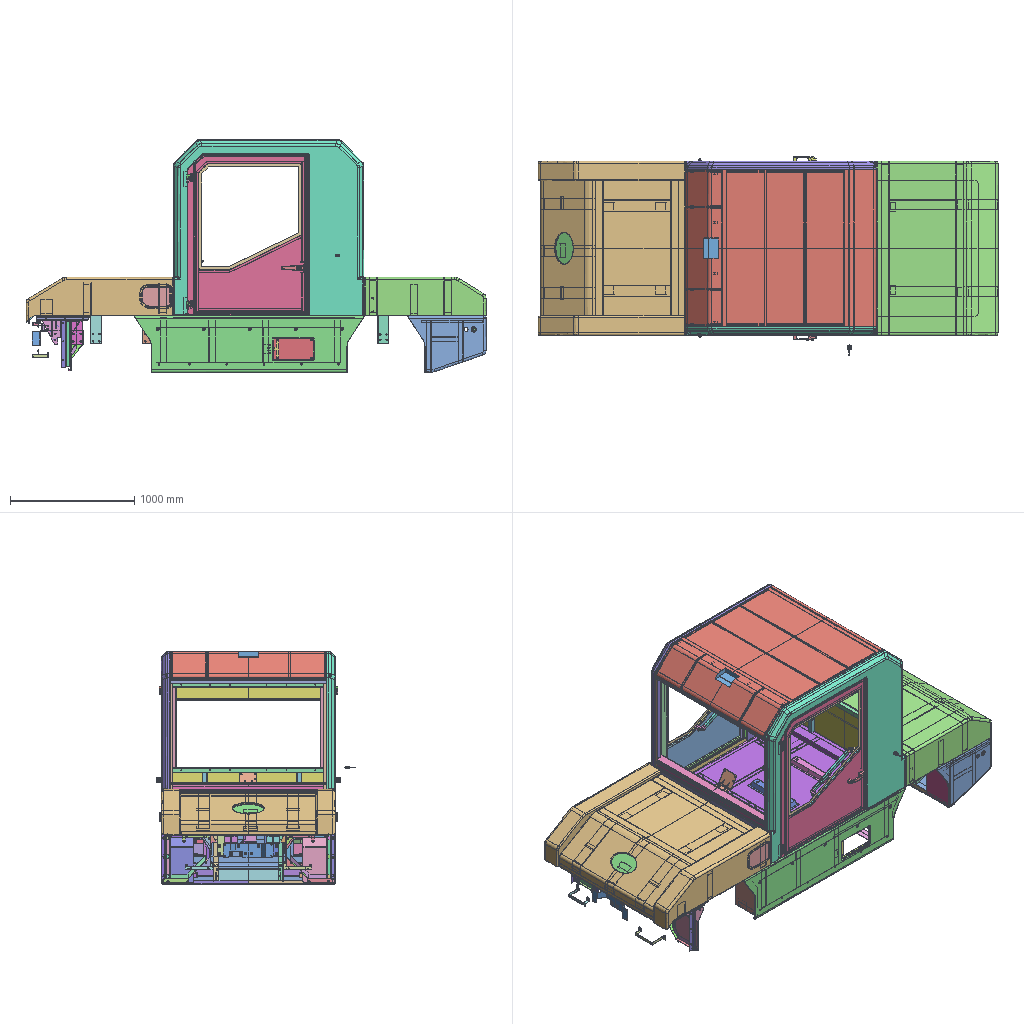Assembly | NX | 146 different items | 266 placed | box 3700 x 1601 x 1871 mm
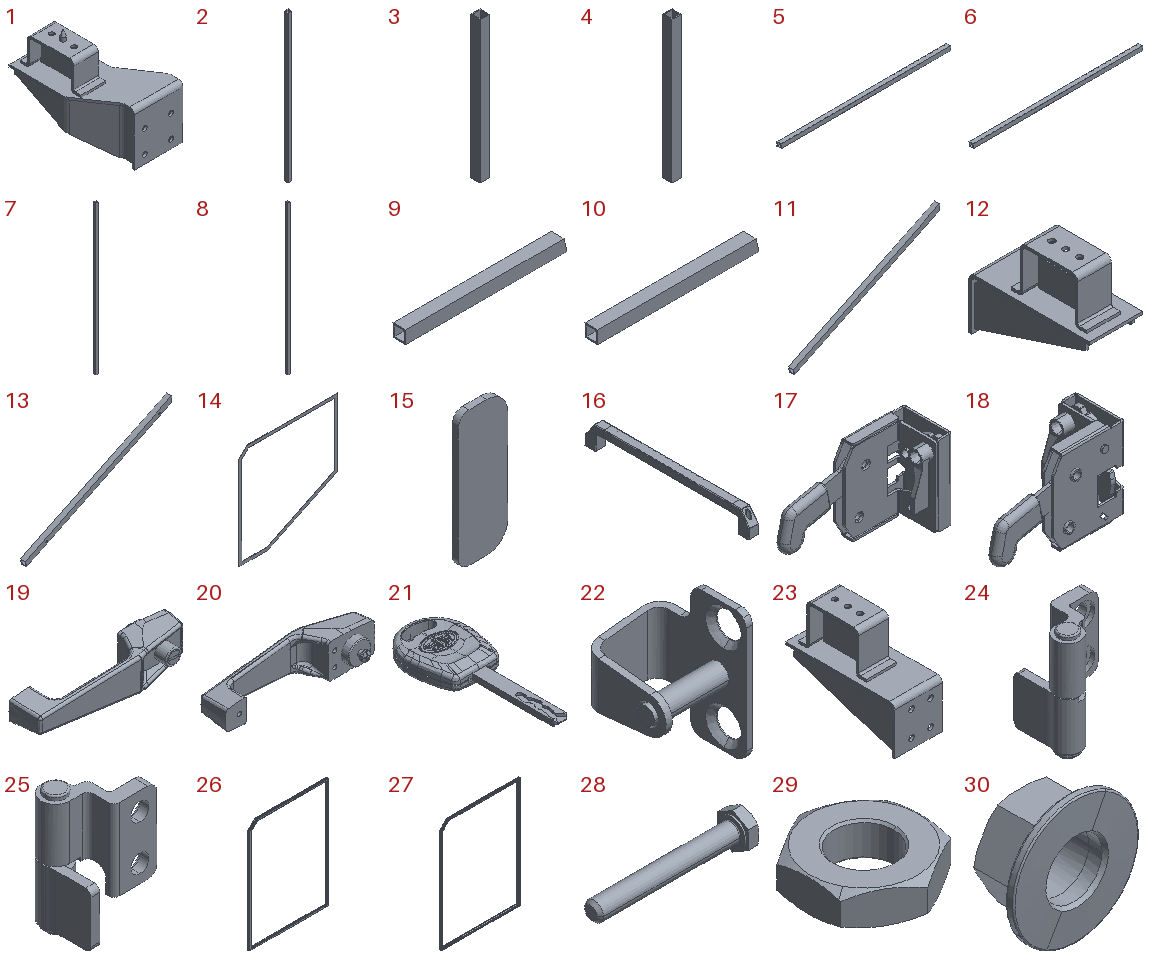Parts list (item | quantity | parent item | size | volume | features):
1 | x1 | in 92 | 193 x 272 x 240 mm | 719296 mm3 | features BREP 7
2 | x1 | in 134 | 20 x 20 x 807.958 mm | 116344 mm3 | features BREP 1
3 | x1 | in 133 | 20 x 20 x 309.106 mm | 44509 mm3 | features BREP 1
4 | x1 | in 134 | 20 x 20 x 309.106 mm | 44509 mm3 | features BREP 1
5 | x1 | in 133 | 830.914 x 20 x 20 mm | 119652 mm3 | features BREP 1
6 | x1 | in 134 | 830.914 x 20 x 20 mm | 119652 mm3 | features BREP 1
7 | x1 | in 133 | - | 161028 mm3 | features BREP 1
8 | x1 | in 134 | 20 x 20 x 1122 mm | 161028 mm3 | features BREP 1
9 | x1 | in 133 | 252.949 x 20 x 20 mm | 36094 mm3 | features BREP 1
10 | x1 | in 134 | 252.949 x 20 x 20 mm | 36094 mm3 | features BREP 1
11 | x1 | in 133 | - | 92693 mm3 | features BREP 1
12 | x1 | in 92 | 114 x 260 x 212 mm | 600917 mm3 | features BREP 6
13 | x1 | in 134 | - | 92693 mm3 | features BREP 1
14 | x2 | in 133, 134 | 830.914 x 2 x 852.689 mm | 150814 mm3 | features BREP 1
15 | x4 | in 133, 134 | - | 4337 mm3 | features BREP 1
16 | x2 | in 135 | 35.311 x 535.2 x 70.2 mm | 135109 mm3 | features BREP 3
17 | x1 | in 135 | 115.249 x 44.6 x 74.6 mm | 46344 mm3 | features BREP 15
18 | x1 | in 135 | - | - | features BREP 15
19 | x1 | in 135 | 184.421 x 56.842 x 42.453 mm | 116707 mm3 | features BREP 1
20 | x1 | in 135 | - | - | features BREP 1
21 | x1 | in 135 | 32.729 x 84.992 x 10.488 mm | 6335 mm3 | features BREP 3
22 | x2 | in 135 | 37 x 44.176 x 60 mm | 11849 mm3 | features BREP 2
23 | x1 | in 92 | 114 x 260 x 212 mm | 600917 mm3 | features BREP 6
24 | x2 | in 135 | 42 x 34.8 x 68 mm | 24506 mm3 | features BREP 6
25 | x2 | in 135 | - | - | features BREP 6
26 | x1 | in 135 | 921.878 x 23.5 x 1292 mm | 1729041 mm3 | features BREP 40
27 | x1 | in 135 | - | - | features BREP 20
28 | x4 | in 135 | 49 x 10 x 11.547 mm | 1597 mm3 | features BREP 1
29 | x8 | in 135 | 13 x 15.011 x 4 mm | 421.241 mm3 | features BREP 1
30 | x6 | in 12, 23, 125 | 26 x 11.959 x 26 mm | 2329 mm3 | features BREP 1
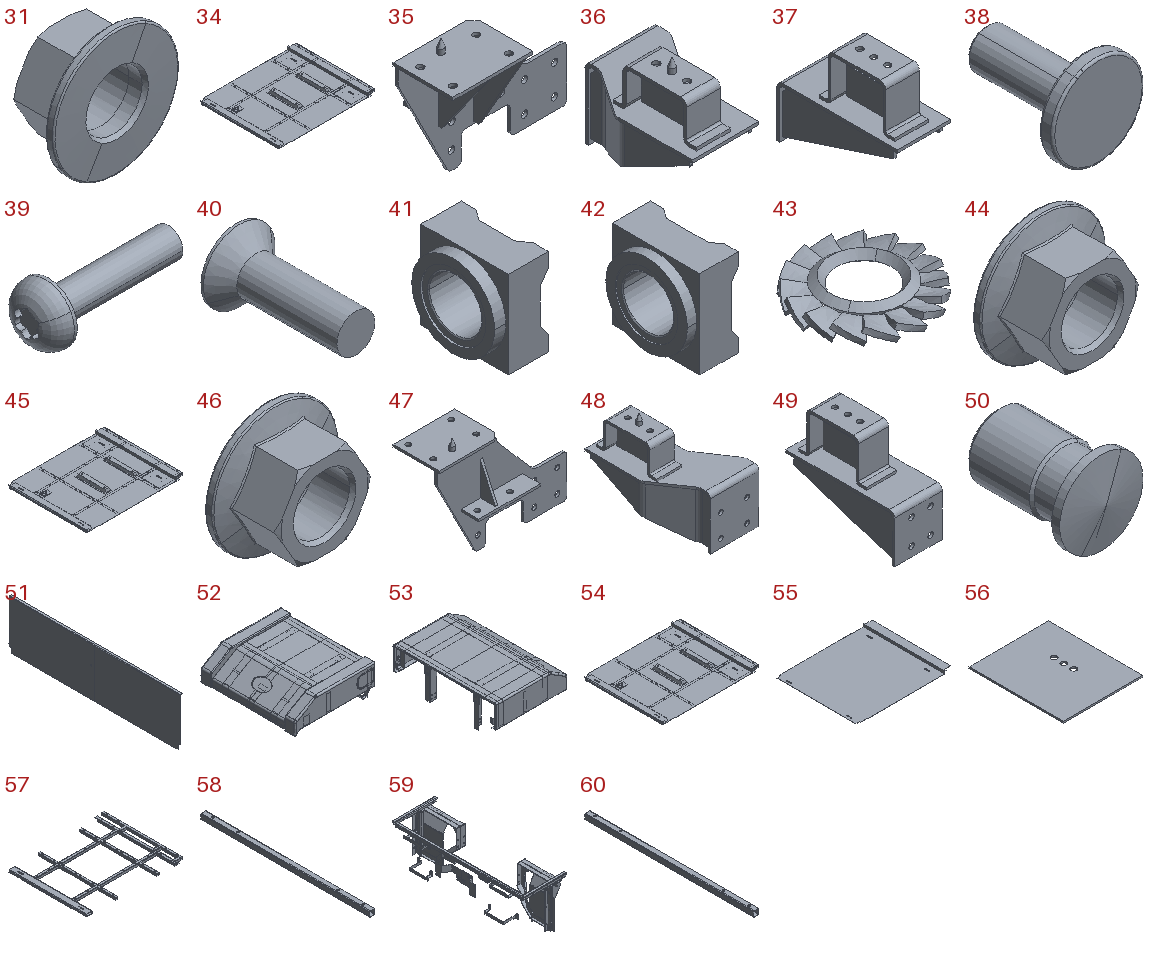31 | x4 | in 114 | 26 x 11.959 x 26 mm | 2329 mm3 | features BREP 1
32 | x1 | in 92 | - | - | -
33 | x1 | in 81 | - | - | -
34 | x1 | in 103 | 1524 x 1300 x 84.135 mm | 9485940 mm3 | features BREP 16
35 | x1 | in 114 | 337.5 x 161 x 259 mm | 536399 mm3 | features BREP 7
36 | x1 | in 125 | 193 x 272 x 240 mm | 714638 mm3 | features BREP 6
37 | x1 | in 12 | 114 x 260 x 212 mm | 596260 mm3 | features BREP 5
38 | x3 | in 73 | 18.5 x 22.7 x 18.5 mm | 1736 mm3 | features BREP 1
39 | x10 | in 135 | 29.6 x 12 x 12 mm | 1095 mm3 | features BREP 1
40 | x4 | in 135 | 15 x 25 x 15 mm | 1509 mm3 | features BREP 1
41 | x4 | in 133, 134 | 5.9 x 10 x 10 mm | 326.565 mm3 | features BREP 1
42 | x14 | in 64, 65, 82, 84, 95, 96, 100 | 7.6 x 14 x 14 mm | 863.218 mm3 | features BREP 1
43 | x4 | in 135 | 16.312 x 16.312 x 2.545 mm | 132.852 mm3 | features BREP 1
44 | x2 | in 1 | 26 x 11.959 x 26 mm | 2329 mm3 | features BREP 1
45 | x1 | in 34 | 1524 x 1300 x 84.135 mm | 9485940 mm3 | features BREP 16
46 | x4 | in 136 | 26 x 11.959 x 26 mm | 2329 mm3 | features BREP 1
47 | x1 | in 136 | 337.5 x 161 x 259 mm | 536399 mm3 | features BREP 7
48 | x1 | in 1 | 193 x 272 x 240 mm | 714638 mm3 | features BREP 6
49 | x1 | in 23 | 114 x 260 x 212 mm | 596260 mm3 | features BREP 5
50 | x8 | in 133, 134 | 10.4 x 13.638 x 10.4 mm | 676.067 mm3 | features BREP 1
51 | x1 | in 84 | 20 x 1258 x 356.004 mm | 935299 mm3 | features BREP 1
52 | x1 | - | 1184 x 1400 x 540.004 mm | 11251128 mm3 | features BREP 91
53 | x1 | - | 983.421 x 1400 x 533.004 mm | 8293382 mm3 | features BREP 71
54 | x1 | in 45 | 1524 x 1300 x 84.135 mm | 9485940 mm3 | features BREP 16
55 | x1 | in 54 | 1516 x 1300 x 44 mm | 4032528 mm3 | features BREP 1
56 | x2 | in 54 | 243.37 x 288 x 5 mm | 347049 mm3 | features BREP 1
57 | x1 | in 54 | 1524 x 1300 x 82 mm | 3863519 mm3 | features BREP 8
58 | x1 | in 57 | 40 x 1258 x 40 mm | 362402 mm3 | features BREP 1
59 | x1 | in 76 | 460.374 x 1390 x 435 mm | 2769143 mm3 | features BREP 60
60 | x1 | in 57 | 40 x 1225 x 40 mm | 352740 mm3 | features BREP 1
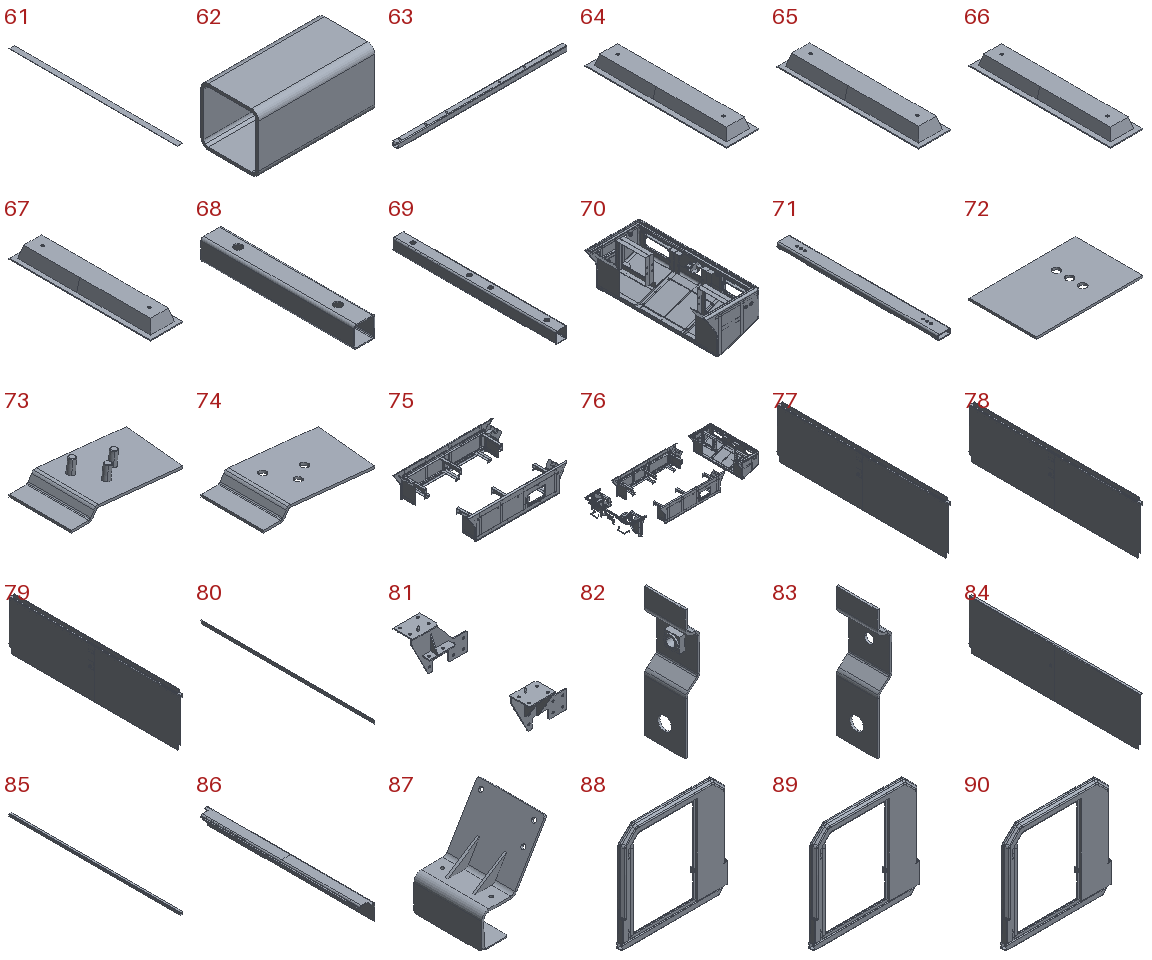61 | x1 | in 57 | 40 x 1300 x 2 mm | 104000 mm3 | features BREP 1
62 | x4 | in 57 | 80.5 x 40 x 40 mm | 23366 mm3 | features BREP 1
63 | x2 | in 57 | 1303 x 40 x 40 mm | 373746 mm3 | features BREP 1
64 | x1 | in 54 | 110 x 481.5 x 37.13 mm | 239621 mm3 | features BREP 2
65 | x1 | in 54 | 110 x 481.5 x 42.13 mm | 251733 mm3 | features BREP 2
66 | x1 | in 64 | 110 x 481.5 x 37.13 mm | 237895 mm3 | features BREP 1
67 | x1 | in 65 | 110 x 481.5 x 42.13 mm | 250007 mm3 | features BREP 1
68 | x4 | in 57 | 40 x 288 x 40 mm | 82180 mm3 | features BREP 1
69 | x2 | in 57 | 40 x 568.999 x 40 mm | 162331 mm3 | features BREP 1
70 | x1 | in 76 | 632.819 x 1400 x 457 mm | 1445450 mm3 | features BREP 93
71 | x1 | in 57 | 100.003 x 1225 x 40 mm | 1550034 mm3 | features BREP 1
72 | x2 | in 54 | 243.374 x 152.848 x 5 mm | 182593 mm3 | features BREP 1
73 | x1 | in 54 | 145.982 x 77.757 x 29.86 mm | 39257 mm3 | features BREP 2
74 | x1 | in 73 | 145.982 x 77.757 x 14.741 mm | 34048 mm3 | features BREP 1
75 | x1 | in 76 | 1856 x 1400 x 457 mm | 7771969 mm3 | features BREP 109
76 | x1 | - | - | 31583893 mm3 | features BREP 278
77 | x1 | in 103 | 28.499 x 1258 x 378.001 mm | 1221396 mm3 | features BREP 5
78 | x1 | in 77 | 28.499 x 1258 x 378.001 mm | 1221396 mm3 | features BREP 5
79 | x1 | in 78 | 28.499 x 1258 x 378.001 mm | 1221396 mm3 | features BREP 5
80 | x1 | in 79 | 4 x 1214 x 21.997 mm | 106850 mm3 | features BREP 1
81 | x1 | in 76 | 337.5 x 830 x 259 mm | 1091429 mm3 | features BREP 16
82 | x1 | in 79 | 14 x 39 x 122.887 mm | 10991 mm3 | features BREP 2
83 | x1 | in 82 | 14 x 39 x 122.887 mm | 10128 mm3 | features BREP 1
84 | x1 | in 79 | 26.5 x 1258 x 356.004 mm | 936162 mm3 | features BREP 2
85 | x1 | in 79 | 20 x 1258 x 20 mm | 167394 mm3 | features BREP 1
86 | x1 | - | 98.003 x 1318 x 131 mm | 1286068 mm3 | features BREP 2
87 | x1 | - | 135.55 x 140 x 179.776 mm | 207099 mm3 | features BREP 2
88 | x1 | in 103 | 1528 x 92.834 x 1503 mm | 9597800 mm3 | features BREP 10
89 | x1 | in 88 | 1528 x 92.834 x 1503 mm | 9597800 mm3 | features BREP 10
90 | x1 | in 89 | 1528 x 92.834 x 1503 mm | 9597800 mm3 | features BREP 10
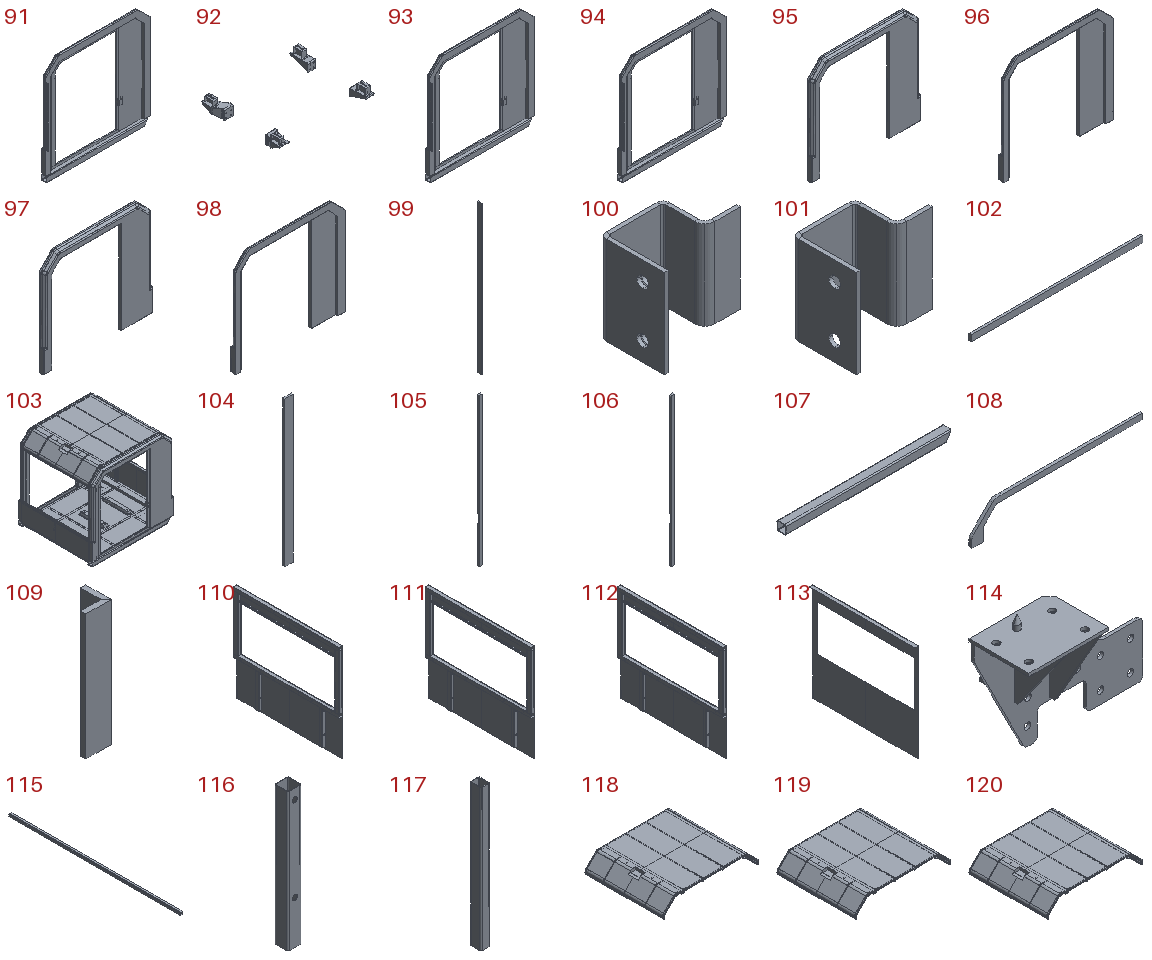91 | x1 | in 103 | 1528 x 92.834 x 1503 mm | 10123824 mm3 | features BREP 10
92 | x1 | - | 1383 x 1144 x 240 mm | 2640420 mm3 | features BREP 24
93 | x1 | in 91 | 1528 x 92.834 x 1503 mm | 10123824 mm3 | features BREP 10
94 | x1 | in 93 | 1528 x 92.834 x 1503 mm | 10123824 mm3 | features BREP 10
95 | x1 | in 90 | 1528 x 70.834 x 1423 mm | 4361637 mm3 | features BREP 2
96 | x1 | in 94 | 1528 x 70.834 x 1423 mm | 4361054 mm3 | features BREP 2
97 | x1 | in 95 | 1528 x 70.834 x 1423 mm | 4357674 mm3 | features BREP 1
98 | x1 | in 96 | 1528 x 70.834 x 1423 mm | 4355566 mm3 | features BREP 1
99 | x2 | in 90, 94 | 4 x 22 x 853.93 mm | 75146 mm3 | features BREP 1
100 | x2 | in 90, 94 | 75 x 50.821 x 70 mm | 32799 mm3 | features BREP 2
101 | x2 | in 100 | 75 x 50.821 x 70 mm | 31072 mm3 | features BREP 1
102 | x2 | in 90, 94 | 977.78 x 15 x 35 mm | 513334 mm3 | features BREP 1
103 | x1 | - | - | 35333668 mm3 | features BREP 44
104 | x2 | in 90, 94 | 65 x 15 x 1103 mm | 1075478 mm3 | features BREP 1
105 | x1 | in 90 | 30 x 15 x 1279 mm | 553706 mm3 | features BREP 1
106 | x2 | in 94 | 30 x 15 x 1279 mm | 553706 mm3 | features BREP 1
107 | x2 | in 90, 94 | 1462 x 80 x 80 mm | 2438141 mm3 | features BREP 1
108 | x2 | in 90, 94 | 947.785 x 15 x 175.635 mm | 489810 mm3 | features BREP 1
109 | x3 | in 90, 94 | 25 x 25 x 125 mm | 28125 mm3 | features BREP 1
110 | x1 | in 103 | 42 x 1260 x 1171 mm | 3345346 mm3 | features BREP 5
111 | x1 | in 110 | 42 x 1260 x 1171 mm | 3345346 mm3 | features BREP 5
112 | x1 | in 111 | 42 x 1260 x 1171 mm | 3345346 mm3 | features BREP 5
113 | x1 | in 112 | 42 x 1258 x 1171 mm | 1789977 mm3 | features BREP 1
114 | x1 | in 81 | 337.5 x 161 x 259 mm | 545714 mm3 | features BREP 8
115 | x1 | in 112 | 20 x 1158 x 20 mm | 150717 mm3 | features BREP 1
116 | x2 | in 112 | 40 x 40 x 404.579 mm | 116022 mm3 | features BREP 1
117 | x2 | in 112 | 40 x 50 x 649.59 mm | 214534 mm3 | features BREP 1
118 | x1 | in 103 | 1528 x 1258 x 253.042 mm | 5712882 mm3 | features BREP 9
119 | x1 | in 118 | 1528 x 1258 x 253.042 mm | 5712882 mm3 | features BREP 9
120 | x1 | in 119 | 1528 x 1258 x 253.042 mm | 5712882 mm3 | features BREP 9
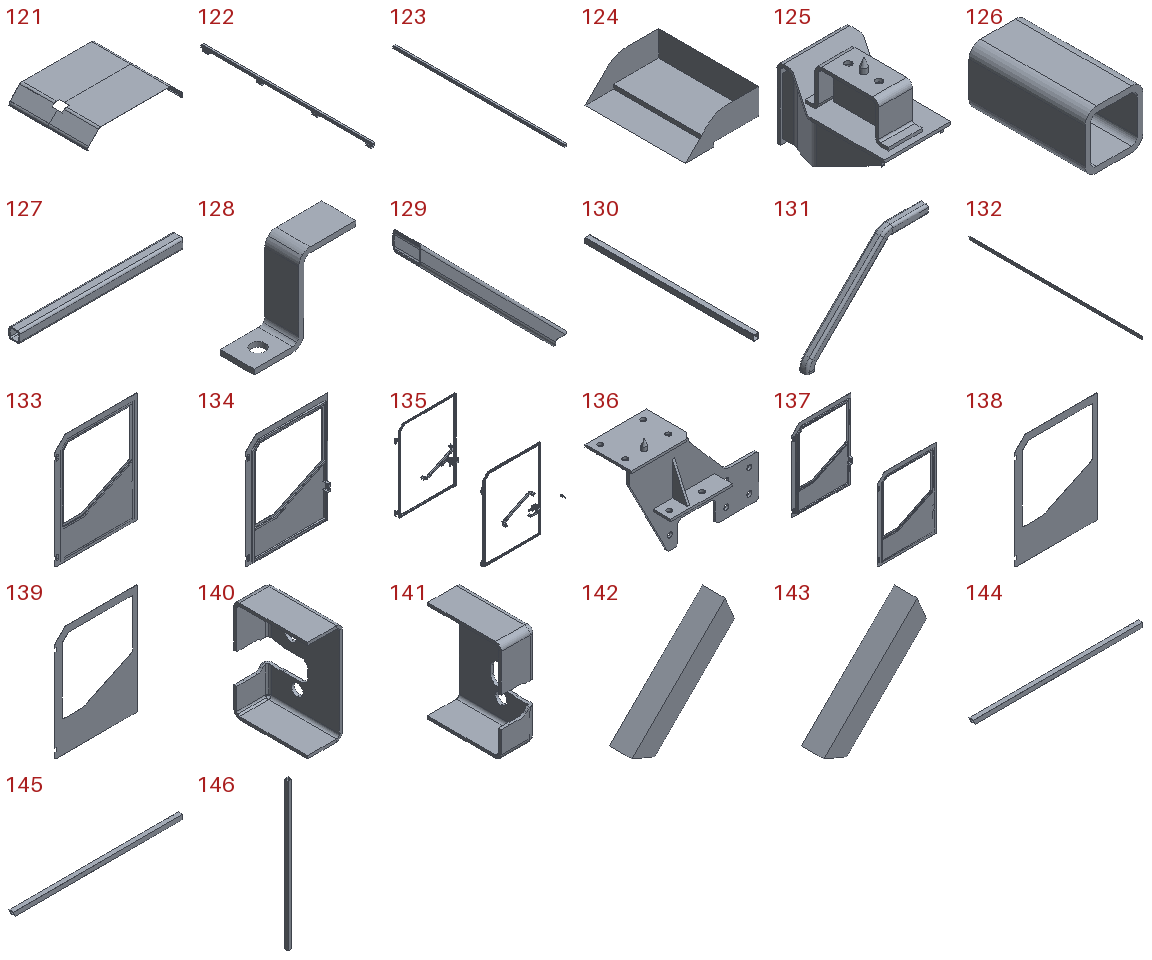121 | x1 | in 120 | 1528 x 1258 x 243.035 mm | 4478605 mm3 | features BREP 1
122 | x2 | in 120 | 20 x 1258 x 40 mm | 188475 mm3 | features BREP 2
123 | x4 | in 120, 122 | 20 x 1258 x 20 mm | 167391 mm3 | features BREP 1
124 | x1 | in 120 | - | - | features BREP 1
125 | x1 | in 92 | 193 x 272 x 240 mm | 719296 mm3 | features BREP 7
126 | x8 | in 122 | 20 x 40 x 20 mm | 5271 mm3 | features BREP 1
127 | x6 | in 120 | 300.997 x 20 x 20 mm | 39934 mm3 | features BREP 1
128 | x4 | in 120 | 49 x 16.34 x 40.003 mm | 3288 mm3 | features BREP 1
129 | x4 | in 120 | 212.69 x 40 x 225.842 mm | 60669 mm3 | features BREP 1
130 | x4 | in 112, 120 | 40 x 1258 x 40 mm | 371774 mm3 | features BREP 1
131 | x4 | in 120 | 286.954 x 20 x 207.051 mm | 47543 mm3 | features BREP 1
132 | x1 | in 120 | 4 x 1258 x 22 mm | 110734 mm3 | features BREP 1
133 | x1 | in 137 | - | 2123684 mm3 | features BREP 14
134 | x1 | in 137 | - | 2123766 mm3 | features BREP 14
135 | x1 | - | - | 1191779 mm3 | features BREP 75
136 | x1 | in 81 | 337.5 x 161 x 259 mm | 545714 mm3 | features BREP 8
137 | x1 | - | - | 4247420 mm3 | features BREP 24
138 | x1 | in 133 | 967.789 x 12 x 1295 mm | 1241371 mm3 | features BREP 1
139 | x1 | in 134 | 967.789 x 2 x 1295 mm | 1241368 mm3 | features BREP 1
140 | x1 | in 133 | - | 23694 mm3 | features BREP 1
141 | x1 | in 134 | 30.233 x 64.001 x 87.693 mm | 23693 mm3 | features BREP 1
142 | x1 | in 133 | - | 15567 mm3 | features BREP 1
143 | x1 | in 134 | 90.584 x 20 x 90.584 mm | 15567 mm3 | features BREP 1
144 | x1 | in 133 | - | 110084 mm3 | features BREP 1
145 | x1 | in 134 | 768.614 x 20 x 20 mm | 110084 mm3 | features BREP 1
146 | x1 | in 133 | 20 x 20 x 807.958 mm | 116344 mm3 | features BREP 1